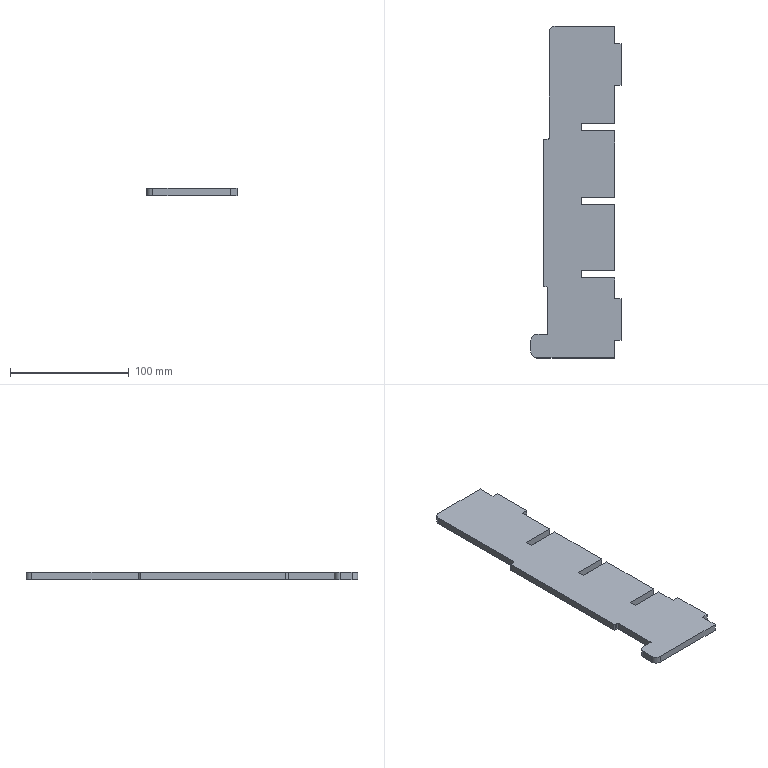Part | SolidWorks | features Fillet 1, FlatPattern 1, SMBaseFlange 1, SheetMetal 1 | 1 solid | 39 faces | box 76 x 280 x 6 mm | volume 97544 mm3 | plane 32 | cylinder 7 | commonest cylinder face diameters 2 x4 10 x3
STEP:
#1=CARTESIAN_POINT('',(-248.5,28.666,0.));
#2=VERTEX_POINT('',#1);
#3=CARTESIAN_POINT('',(-249.5,27.666,0.));
#4=VERTEX_POINT('',#3);
#5=CARTESIAN_POINT('',(-248.5,27.666,0.));
#6=DIRECTION('',(0.,0.,1.));
#7=DIRECTION('',(1.,0.,0.));
#8=AXIS2_PLACEMENT_3D('',#5,#6,#7);
#9=CIRCLE('',#8,1.);
#10=EDGE_CURVE('',#2,#4,#9,.T.);
#11=ORIENTED_EDGE('',*,*,#10,.F.);
#12=CARTESIAN_POINT('',(-248.5,28.666,-6.));
#13=VERTEX_POINT('',#12);
#14=CARTESIAN_POINT('',(-248.5,28.666,-6.));
#15=DIRECTION('',(0.,0.,1.));
#16=VECTOR('',#15,1000.);
#17=LINE('',#14,#16);
#18=EDGE_CURVE('',#13,#2,#17,.T.);
#19=ORIENTED_EDGE('',*,*,#18,.F.);
#20=CARTESIAN_POINT('',(-249.5,27.666,-6.));
#21=VERTEX_POINT('',#20);
#22=CARTESIAN_POINT('',(-248.5,27.666,-6.));
#23=DIRECTION('',(0.,0.,1.));
#24=DIRECTION('',(1.,0.,0.));
#25=AXIS2_PLACEMENT_3D('',#22,#23,#24);
#26=CIRCLE('',#25,1.);
#27=EDGE_CURVE('',#13,#21,#26,.T.);
#28=ORIENTED_EDGE('',*,*,#27,.T.);
#29=CARTESIAN_POINT('',(-249.5,27.666,-6.));
#30=DIRECTION('',(0.,0.,1.));
#31=VECTOR('',#30,1000.);
#32=LINE('',#29,#31);
#33=EDGE_CURVE('',#21,#4,#32,.T.);
#34=ORIENTED_EDGE('',*,*,#33,.T.);
#35=EDGE_LOOP('',(#11,#19,#28,#34));
#36=FACE_OUTER_BOUND('',#35,.T.);
#37=CARTESIAN_POINT('',(-248.5,27.666,-6.));
#38=DIRECTION('',(0.,0.,1.));
#39=DIRECTION('',(1.,0.,0.));
#40=AXIS2_PLACEMENT_3D('',#37,#38,#39);
#41=CYLINDRICAL_SURFACE('',#40,1.);
#42=ADVANCED_FACE('',(#36),#41,.T.);
#43=CARTESIAN_POINT('',(-245.5,28.666,0.));
#44=VERTEX_POINT('',#43);
#45=CARTESIAN_POINT('',(-248.5,28.666,0.));
#46=DIRECTION('',(-1.,0.,0.));
#47=VECTOR('',#46,1000.);
#48=LINE('',#45,#47);
#49=EDGE_CURVE('',#44,#2,#48,.T.);
#50=ORIENTED_EDGE('',*,*,#49,.F.);
#51=CARTESIAN_POINT('',(-245.5,28.666,-6.));
#52=VERTEX_POINT('',#51);
#53=CARTESIAN_POINT('',(-245.5,28.666,-6.));
#54=DIRECTION('',(0.,0.,1.));
#55=VECTOR('',#54,1000.);
#56=LINE('',#53,#55);
#57=EDGE_CURVE('',#52,#44,#56,.T.);
#58=ORIENTED_EDGE('',*,*,#57,.F.);
#59=CARTESIAN_POINT('',(-248.5,28.666,-6.));
#60=DIRECTION('',(-1.,0.,0.));
#61=VECTOR('',#60,1000.);
#62=LINE('',#59,#61);
#63=EDGE_CURVE('',#52,#13,#62,.T.);
#64=ORIENTED_EDGE('',*,*,#63,.T.);
#65=ORIENTED_EDGE('',*,*,#18,.T.);
#66=EDGE_LOOP('',(#50,#58,#64,#65));
#67=FACE_OUTER_BOUND('',#66,.T.);
#68=CARTESIAN_POINT('',(-248.5,28.666,-6.));
#69=DIRECTION('',(0.,1.,0.));
#70=DIRECTION('',(0.,0.,1.));
#71=AXIS2_PLACEMENT_3D('',#68,#69,#70);
#72=PLANE('',#71);
#73=ADVANCED_FACE('',(#67),#72,.T.);
#74=CARTESIAN_POINT('',(-244.5,29.666,0.));
#75=VERTEX_POINT('',#74);
#76=CARTESIAN_POINT('',(-245.5,29.666,0.));
#77=DIRECTION('',(0.,0.,-1.));
#78=DIRECTION('',(1.,0.,0.));
#79=AXIS2_PLACEMENT_3D('',#76,#77,#78);
#80=CIRCLE('',#79,1.);
#81=EDGE_CURVE('',#75,#44,#80,.T.);
#82=ORIENTED_EDGE('',*,*,#81,.F.);
#83=CARTESIAN_POINT('',(-244.5,29.666,-6.));
#84=VERTEX_POINT('',#83);
#85=CARTESIAN_POINT('',(-244.5,29.666,-6.));
#86=DIRECTION('',(0.,0.,1.));
#87=VECTOR('',#86,1000.);
#88=LINE('',#85,#87);
#89=EDGE_CURVE('',#84,#75,#88,.T.);
#90=ORIENTED_EDGE('',*,*,#89,.F.);
#91=CARTESIAN_POINT('',(-245.5,29.666,-6.));
#92=DIRECTION('',(0.,0.,-1.));
#93=DIRECTION('',(1.,0.,0.));
#94=AXIS2_PLACEMENT_3D('',#91,#92,#93);
#95=CIRCLE('',#94,1.);
#96=EDGE_CURVE('',#84,#52,#95,.T.);
#97=ORIENTED_EDGE('',*,*,#96,.T.);
#98=ORIENTED_EDGE('',*,*,#57,.T.);
#99=EDGE_LOOP('',(#82,#90,#97,#98));
#100=FACE_OUTER_BOUND('',#99,.T.);
#101=CARTESIAN_POINT('',(-245.5,29.666,-6.));
#102=DIRECTION('',(0.,0.,1.));
#103=DIRECTION('',(1.,0.,0.));
#104=AXIS2_PLACEMENT_3D('',#101,#102,#103);
#105=CYLINDRICAL_SURFACE('',#104,1.);
#106=ADVANCED_FACE('',(#100),#105,.F.);
#107=CARTESIAN_POINT('',(-244.5,119.166,0.));
#108=VERTEX_POINT('',#107);
#109=CARTESIAN_POINT('',(-244.5,124.166,0.));
#110=DIRECTION('',(0.,-1.,0.));
#111=VECTOR('',#110,1000.);
#112=LINE('',#109,#111);
#113=EDGE_CURVE('',#108,#75,#112,.T.);
#114=ORIENTED_EDGE('',*,*,#113,.F.);
#115=CARTESIAN_POINT('',(-244.5,119.166,-6.));
#116=VERTEX_POINT('',#115);
#117=CARTESIAN_POINT('',(-244.5,119.166,-6.));
#118=DIRECTION('',(0.,0.,-1.));
#119=VECTOR('',#118,1000.);
#120=LINE('',#117,#119);
#121=EDGE_CURVE('',#108,#116,#120,.T.);
#122=ORIENTED_EDGE('',*,*,#121,.T.);
#123=CARTESIAN_POINT('',(-244.5,124.166,-6.));
#124=DIRECTION('',(0.,-1.,0.));
#125=VECTOR('',#124,1000.);
#126=LINE('',#123,#125);
#127=EDGE_CURVE('',#116,#84,#126,.T.);
#128=ORIENTED_EDGE('',*,*,#127,.T.);
#129=ORIENTED_EDGE('',*,*,#89,.T.);
#130=EDGE_LOOP('',(#114,#122,#128,#129));
#131=FACE_OUTER_BOUND('',#130,.T.);
#132=CARTESIAN_POINT('',(-244.5,124.166,-6.));
#133=DIRECTION('',(-1.,0.,0.));
#134=DIRECTION('',(0.,-1.,0.));
#135=AXIS2_PLACEMENT_3D('',#132,#133,#134);
#136=PLANE('',#135);
#137=ADVANCED_FACE('',(#131),#136,.T.);
#138=CARTESIAN_POINT('',(-189.5,124.166,-6.));
#139=VERTEX_POINT('',#138);
#140=CARTESIAN_POINT('',(-239.5,124.166,-6.));
#141=VERTEX_POINT('',#140);
#142=CARTESIAN_POINT('',(-189.5,124.166,-6.));
#143=DIRECTION('',(-1.,0.,0.));
#144=VECTOR('',#143,1000.);
#145=LINE('',#142,#144);
#146=EDGE_CURVE('',#139,#141,#145,.T.);
#147=ORIENTED_EDGE('',*,*,#146,.T.);
#148=CARTESIAN_POINT('',(-239.5,124.166,0.));
#149=VERTEX_POINT('',#148);
#150=CARTESIAN_POINT('',(-239.5,124.166,-6.));
#151=DIRECTION('',(0.,0.,1.));
#152=VECTOR('',#151,1000.);
#153=LINE('',#150,#152);
#154=EDGE_CURVE('',#141,#149,#153,.T.);
#155=ORIENTED_EDGE('',*,*,#154,.T.);
#156=CARTESIAN_POINT('',(-189.5,124.166,0.));
#157=VERTEX_POINT('',#156);
#158=CARTESIAN_POINT('',(-189.5,124.166,0.));
#159=DIRECTION('',(-1.,0.,0.));
#160=VECTOR('',#159,1000.);
#161=LINE('',#158,#160);
#162=EDGE_CURVE('',#157,#149,#161,.T.);
#163=ORIENTED_EDGE('',*,*,#162,.F.);
#164=CARTESIAN_POINT('',(-189.5,124.166,-6.));
#165=DIRECTION('',(0.,0.,1.));
#166=VECTOR('',#165,1000.);
#167=LINE('',#164,#166);
#168=EDGE_CURVE('',#139,#157,#167,.T.);
#169=ORIENTED_EDGE('',*,*,#168,.F.);
#170=EDGE_LOOP('',(#147,#155,#163,#169));
#171=FACE_OUTER_BOUND('',#170,.T.);
#172=CARTESIAN_POINT('',(-189.5,124.166,-6.));
#173=DIRECTION('',(0.,1.,0.));
#174=DIRECTION('',(0.,0.,1.));
#175=AXIS2_PLACEMENT_3D('',#172,#173,#174);
#176=PLANE('',#175);
#177=ADVANCED_FACE('',(#171),#176,.T.);
#178=CARTESIAN_POINT('',(-189.5,109.166,0.));
#179=VERTEX_POINT('',#178);
#180=CARTESIAN_POINT('',(-189.5,109.166,0.));
#181=DIRECTION('',(0.,1.,0.));
#182=VECTOR('',#181,1000.);
#183=LINE('',#180,#182);
#184=EDGE_CURVE('',#179,#157,#183,.T.);
#185=ORIENTED_EDGE('',*,*,#184,.F.);
#186=CARTESIAN_POINT('',(-189.5,109.166,-6.));
#187=VERTEX_POINT('',#186);
#188=CARTESIAN_POINT('',(-189.5,109.166,-6.));
#189=DIRECTION('',(0.,0.,1.));
#190=VECTOR('',#189,1000.);
#191=LINE('',#188,#190);
#192=EDGE_CURVE('',#187,#179,#191,.T.);
#193=ORIENTED_EDGE('',*,*,#192,.F.);
#194=CARTESIAN_POINT('',(-189.5,109.166,-6.));
#195=DIRECTION('',(0.,1.,0.));
#196=VECTOR('',#195,1000.);
#197=LINE('',#194,#196);
#198=EDGE_CURVE('',#187,#139,#197,.T.);
#199=ORIENTED_EDGE('',*,*,#198,.T.);
#200=ORIENTED_EDGE('',*,*,#168,.T.);
#201=EDGE_LOOP('',(#185,#193,#199,#200));
#202=FACE_OUTER_BOUND('',#201,.T.);
#203=CARTESIAN_POINT('',(-189.5,109.166,-6.));
#204=DIRECTION('',(1.,0.,0.));
#205=DIRECTION('',(0.,1.,0.));
#206=AXIS2_PLACEMENT_3D('',#203,#204,#205);
#207=PLANE('',#206);
#208=ADVANCED_FACE('',(#202),#207,.T.);
#209=CARTESIAN_POINT('',(-184.,109.166,0.));
#210=VERTEX_POINT('',#209);
#211=CARTESIAN_POINT('',(-189.5,109.166,0.));
#212=DIRECTION('',(-1.,0.,0.));
#213=VECTOR('',#212,1000.);
#214=LINE('',#211,#213);
#215=EDGE_CURVE('',#210,#179,#214,.T.);
#216=ORIENTED_EDGE('',*,*,#215,.F.);
#217=CARTESIAN_POINT('',(-184.,109.166,-6.));
#218=VERTEX_POINT('',#217);
#219=CARTESIAN_POINT('',(-184.,109.166,-6.));
#220=DIRECTION('',(0.,0.,1.));
#221=VECTOR('',#220,1000.);
#222=LINE('',#219,#221);
#223=EDGE_CURVE('',#218,#210,#222,.T.);
#224=ORIENTED_EDGE('',*,*,#223,.F.);
#225=CARTESIAN_POINT('',(-189.5,109.166,-6.));
#226=DIRECTION('',(-1.,0.,0.));
#227=VECTOR('',#226,1000.);
#228=LINE('',#225,#227);
#229=EDGE_CURVE('',#218,#187,#228,.T.);
#230=ORIENTED_EDGE('',*,*,#229,.T.);
#231=ORIENTED_EDGE('',*,*,#192,.T.);
#232=EDGE_LOOP('',(#216,#224,#230,#231));
#233=FACE_OUTER_BOUND('',#232,.T.);
#234=CARTESIAN_POINT('',(-189.5,109.166,-6.));
#235=DIRECTION('',(0.,1.,0.));
#236=DIRECTION('',(0.,0.,1.));
#237=AXIS2_PLACEMENT_3D('',#234,#235,#236);
#238=PLANE('',#237);
#239=ADVANCED_FACE('',(#233),#238,.T.);
#240=CARTESIAN_POINT('',(-184.,74.166,0.));
#241=VERTEX_POINT('',#240);
#242=CARTESIAN_POINT('',(-184.,109.166,0.));
#243=DIRECTION('',(0.,1.,0.));
#244=VECTOR('',#243,1000.);
#245=LINE('',#242,#244);
#246=EDGE_CURVE('',#241,#210,#245,.T.);
#247=ORIENTED_EDGE('',*,*,#246,.F.);
#248=CARTESIAN_POINT('',(-184.,74.166,-6.));
#249=VERTEX_POINT('',#248);
#250=CARTESIAN_POINT('',(-184.,74.166,-6.));
#251=DIRECTION('',(0.,0.,1.));
#252=VECTOR('',#251,1000.);
#253=LINE('',#250,#252);
#254=EDGE_CURVE('',#249,#241,#253,.T.);
#255=ORIENTED_EDGE('',*,*,#254,.F.);
#256=CARTESIAN_POINT('',(-184.,109.166,-6.));
#257=DIRECTION('',(0.,1.,0.));
#258=VECTOR('',#257,1000.);
#259=LINE('',#256,#258);
#260=EDGE_CURVE('',#249,#218,#259,.T.);
#261=ORIENTED_EDGE('',*,*,#260,.T.);
#262=ORIENTED_EDGE('',*,*,#223,.T.);
#263=EDGE_LOOP('',(#247,#255,#261,#262));
#264=FACE_OUTER_BOUND('',#263,.T.);
#265=CARTESIAN_POINT('',(-184.,109.166,-6.));
#266=DIRECTION('',(1.,0.,0.));
#267=DIRECTION('',(0.,0.,-1.));
#268=AXIS2_PLACEMENT_3D('',#265,#266,#267);
#269=PLANE('',#268);
#270=ADVANCED_FACE('',(#264),#269,.T.);
#271=CARTESIAN_POINT('',(-189.5,74.166,0.));
#272=VERTEX_POINT('',#271);
#273=CARTESIAN_POINT('',(-184.,74.166,0.));
#274=DIRECTION('',(1.,0.,0.));
#275=VECTOR('',#274,1000.);
#276=LINE('',#273,#275);
#277=EDGE_CURVE('',#272,#241,#276,.T.);
#278=ORIENTED_EDGE('',*,*,#277,.F.);
#279=CARTESIAN_POINT('',(-189.5,74.166,-6.));
#280=VERTEX_POINT('',#279);
#281=CARTESIAN_POINT('',(-189.5,74.166,-6.));
#282=DIRECTION('',(0.,0.,1.));
#283=VECTOR('',#282,1000.);
#284=LINE('',#281,#283);
#285=EDGE_CURVE('',#280,#272,#284,.T.);
#286=ORIENTED_EDGE('',*,*,#285,.F.);
#287=CARTESIAN_POINT('',(-184.,74.166,-6.));
#288=DIRECTION('',(1.,0.,0.));
#289=VECTOR('',#288,1000.);
#290=LINE('',#287,#289);
#291=EDGE_CURVE('',#280,#249,#290,.T.);
#292=ORIENTED_EDGE('',*,*,#291,.T.);
#293=ORIENTED_EDGE('',*,*,#254,.T.);
#294=EDGE_LOOP('',(#278,#286,#292,#293));
#295=FACE_OUTER_BOUND('',#294,.T.);
#296=CARTESIAN_POINT('',(-184.,74.166,-6.));
#297=DIRECTION('',(0.,-1.,0.));
#298=DIRECTION('',(0.,0.,-1.));
#299=AXIS2_PLACEMENT_3D('',#296,#297,#298);
#300=PLANE('',#299);
#301=ADVANCED_FACE('',(#295),#300,.T.);
#302=CARTESIAN_POINT('',(-189.5,41.666,0.));
#303=VERTEX_POINT('',#302);
#304=CARTESIAN_POINT('',(-189.5,41.666,0.));
#305=DIRECTION('',(0.,1.,0.));
#306=VECTOR('',#305,1000.);
#307=LINE('',#304,#306);
#308=EDGE_CURVE('',#303,#272,#307,.T.);
#309=ORIENTED_EDGE('',*,*,#308,.F.);
#310=CARTESIAN_POINT('',(-189.5,41.666,-6.));
#311=VERTEX_POINT('',#310);
#312=CARTESIAN_POINT('',(-189.5,41.666,-6.));
#313=DIRECTION('',(0.,0.,1.));
#314=VECTOR('',#313,1000.);
#315=LINE('',#312,#314);
#316=EDGE_CURVE('',#311,#303,#315,.T.);
#317=ORIENTED_EDGE('',*,*,#316,.F.);
#318=CARTESIAN_POINT('',(-189.5,41.666,-6.));
#319=DIRECTION('',(0.,1.,0.));
#320=VECTOR('',#319,1000.);
#321=LINE('',#318,#320);
#322=EDGE_CURVE('',#311,#280,#321,.T.);
#323=ORIENTED_EDGE('',*,*,#322,.T.);
#324=ORIENTED_EDGE('',*,*,#285,.T.);
#325=EDGE_LOOP('',(#309,#317,#323,#324));
#326=FACE_OUTER_BOUND('',#325,.T.);
#327=CARTESIAN_POINT('',(-189.5,41.666,-6.));
#328=DIRECTION('',(1.,0.,0.));
#329=DIRECTION('',(0.,1.,0.));
#330=AXIS2_PLACEMENT_3D('',#327,#328,#329);
#331=PLANE('',#330);
#332=ADVANCED_FACE('',(#326),#331,.T.);
#333=CARTESIAN_POINT('',(-217.5,41.666,0.));
#334=VERTEX_POINT('',#333);
#335=CARTESIAN_POINT('',(-217.5,41.666,0.));
#336=DIRECTION('',(1.,0.,0.));
#337=VECTOR('',#336,1000.);
#338=LINE('',#335,#337);
#339=EDGE_CURVE('',#334,#303,#338,.T.);
#340=ORIENTED_EDGE('',*,*,#339,.F.);
#341=CARTESIAN_POINT('',(-217.5,41.666,-6.));
#342=VERTEX_POINT('',#341);
#343=CARTESIAN_POINT('',(-217.5,41.666,-6.));
#344=DIRECTION('',(0.,0.,1.));
#345=VECTOR('',#344,1000.);
#346=LINE('',#343,#345);
#347=EDGE_CURVE('',#342,#334,#346,.T.);
#348=ORIENTED_EDGE('',*,*,#347,.F.);
#349=CARTESIAN_POINT('',(-217.5,41.666,-6.));
#350=DIRECTION('',(1.,0.,0.));
#351=VECTOR('',#350,1000.);
#352=LINE('',#349,#351);
#353=EDGE_CURVE('',#342,#311,#352,.T.);
#354=ORIENTED_EDGE('',*,*,#353,.T.);
#355=ORIENTED_EDGE('',*,*,#316,.T.);
#356=EDGE_LOOP('',(#340,#348,#354,#355));
#357=FACE_OUTER_BOUND('',#356,.T.);
#358=CARTESIAN_POINT('',(-217.5,41.666,-6.));
#359=DIRECTION('',(0.,-1.,0.));
#360=DIRECTION('',(1.,0.,0.));
#361=AXIS2_PLACEMENT_3D('',#358,#359,#360);
#362=PLANE('',#361);
#363=ADVANCED_FACE('',(#357),#362,.T.);
#364=CARTESIAN_POINT('',(-217.5,35.666,0.));
#365=VERTEX_POINT('',#364);
#366=CARTESIAN_POINT('',(-217.5,35.666,0.));
#367=DIRECTION('',(0.,1.,0.));
#368=VECTOR('',#367,1000.);
#369=LINE('',#366,#368);
#370=EDGE_CURVE('',#365,#334,#369,.T.);
#371=ORIENTED_EDGE('',*,*,#370,.F.);
#372=CARTESIAN_POINT('',(-217.5,35.666,-6.));
#373=VERTEX_POINT('',#372);
#374=CARTESIAN_POINT('',(-217.5,35.666,-6.));
#375=DIRECTION('',(0.,0.,1.));
#376=VECTOR('',#375,1000.);
#377=LINE('',#374,#376);
#378=EDGE_CURVE('',#373,#365,#377,.T.);
#379=ORIENTED_EDGE('',*,*,#378,.F.);
#380=CARTESIAN_POINT('',(-217.5,35.666,-6.));
#381=DIRECTION('',(0.,1.,0.));
#382=VECTOR('',#381,1000.);
#383=LINE('',#380,#382);
#384=EDGE_CURVE('',#373,#342,#383,.T.);
#385=ORIENTED_EDGE('',*,*,#384,.T.);
#386=ORIENTED_EDGE('',*,*,#347,.T.);
#387=EDGE_LOOP('',(#371,#379,#385,#386));
#388=FACE_OUTER_BOUND('',#387,.T.);
#389=CARTESIAN_POINT('',(-217.5,35.666,-6.));
#390=DIRECTION('',(1.,0.,0.));
#391=DIRECTION('',(0.,0.,-1.));
#392=AXIS2_PLACEMENT_3D('',#389,#390,#391);
#393=PLANE('',#392);
#394=ADVANCED_FACE('',(#388),#393,.T.);
#395=CARTESIAN_POINT('',(-189.5,35.666,0.));
#396=VERTEX_POINT('',#395);
#397=CARTESIAN_POINT('',(-189.5,35.666,0.));
#398=DIRECTION('',(-1.,0.,0.));
#399=VECTOR('',#398,1000.);
#400=LINE('',#397,#399);
#401=EDGE_CURVE('',#396,#365,#400,.T.);
#402=ORIENTED_EDGE('',*,*,#401,.F.);
#403=CARTESIAN_POINT('',(-189.5,35.666,-6.));
#404=VERTEX_POINT('',#403);
#405=CARTESIAN_POINT('',(-189.5,35.666,-6.));
#406=DIRECTION('',(0.,0.,1.));
#407=VECTOR('',#406,1000.);
#408=LINE('',#405,#407);
#409=EDGE_CURVE('',#404,#396,#408,.T.);
#410=ORIENTED_EDGE('',*,*,#409,.F.);
#411=CARTESIAN_POINT('',(-189.5,35.666,-6.));
#412=DIRECTION('',(-1.,0.,0.));
#413=VECTOR('',#412,1000.);
#414=LINE('',#411,#413);
#415=EDGE_CURVE('',#404,#373,#414,.T.);
#416=ORIENTED_EDGE('',*,*,#415,.T.);
#417=ORIENTED_EDGE('',*,*,#378,.T.);
#418=EDGE_LOOP('',(#402,#410,#416,#417));
#419=FACE_OUTER_BOUND('',#418,.T.);
#420=CARTESIAN_POINT('',(-189.5,35.666,-6.));
#421=DIRECTION('',(0.,1.,0.));
#422=DIRECTION('',(-1.,0.,0.));
#423=AXIS2_PLACEMENT_3D('',#420,#421,#422);
#424=PLANE('',#423);
#425=ADVANCED_FACE('',(#419),#424,.T.);
#426=CARTESIAN_POINT('',(-189.5,-20.334,0.));
#427=VERTEX_POINT('',#426);
#428=CARTESIAN_POINT('',(-189.5,-20.334,0.));
#429=DIRECTION('',(0.,1.,0.));
#430=VECTOR('',#429,1000.);
#431=LINE('',#428,#430);
#432=EDGE_CURVE('',#427,#396,#431,.T.);
#433=ORIENTED_EDGE('',*,*,#432,.F.);
#434=CARTESIAN_POINT('',(-189.5,-20.334,-6.));
#435=VERTEX_POINT('',#434);
#436=CARTESIAN_POINT('',(-189.5,-20.334,-6.));
#437=DIRECTION('',(0.,0.,1.));
#438=VECTOR('',#437,1000.);
#439=LINE('',#436,#438);
#440=EDGE_CURVE('',#435,#427,#439,.T.);
#441=ORIENTED_EDGE('',*,*,#440,.F.);
#442=CARTESIAN_POINT('',(-189.5,-20.334,-6.));
#443=DIRECTION('',(0.,1.,0.));
#444=VECTOR('',#443,1000.);
#445=LINE('',#442,#444);
#446=EDGE_CURVE('',#435,#404,#445,.T.);
#447=ORIENTED_EDGE('',*,*,#446,.T.);
#448=ORIENTED_EDGE('',*,*,#409,.T.);
#449=EDGE_LOOP('',(#433,#441,#447,#448));
#450=FACE_OUTER_BOUND('',#449,.T.);
#451=CARTESIAN_POINT('',(-189.5,-20.334,-6.));
#452=DIRECTION('',(1.,0.,0.));
#453=DIRECTION('',(0.,0.,-1.));
#454=AXIS2_PLACEMENT_3D('',#451,#452,#453);
#455=PLANE('',#454);
#456=ADVANCED_FACE('',(#450),#455,.T.);
#457=CARTESIAN_POINT('',(-217.5,-20.334,0.));
#458=VERTEX_POINT('',#457);
#459=CARTESIAN_POINT('',(-217.5,-20.334,0.));
#460=DIRECTION('',(1.,0.,0.));
#461=VECTOR('',#460,1000.);
#462=LINE('',#459,#461);
#463=EDGE_CURVE('',#458,#427,#462,.T.);
#464=ORIENTED_EDGE('',*,*,#463,.F.);
#465=CARTESIAN_POINT('',(-217.5,-20.334,-6.));
#466=VERTEX_POINT('',#465);
#467=CARTESIAN_POINT('',(-217.5,-20.334,-6.));
#468=DIRECTION('',(0.,0.,1.));
#469=VECTOR('',#468,1000.);
#470=LINE('',#467,#469);
#471=EDGE_CURVE('',#466,#458,#470,.T.);
#472=ORIENTED_EDGE('',*,*,#471,.F.);
#473=CARTESIAN_POINT('',(-217.5,-20.334,-6.));
#474=DIRECTION('',(1.,0.,0.));
#475=VECTOR('',#474,1000.);
#476=LINE('',#473,#475);
#477=EDGE_CURVE('',#466,#435,#476,.T.);
#478=ORIENTED_EDGE('',*,*,#477,.T.);
#479=ORIENTED_EDGE('',*,*,#440,.T.);
#480=EDGE_LOOP('',(#464,#472,#478,#479));
#481=FACE_OUTER_BOUND('',#480,.T.);
#482=CARTESIAN_POINT('',(-217.5,-20.334,-6.));
#483=DIRECTION('',(0.,-1.,0.));
#484=DIRECTION('',(1.,0.,0.));
#485=AXIS2_PLACEMENT_3D('',#482,#483,#484);
#486=PLANE('',#485);
#487=ADVANCED_FACE('',(#481),#486,.T.);
#488=CARTESIAN_POINT('',(-217.5,-26.334,0.));
#489=VERTEX_POINT('',#488);
#490=CARTESIAN_POINT('',(-217.5,-26.334,0.));
#491=DIRECTION('',(0.,1.,0.));
#492=VECTOR('',#491,1000.);
#493=LINE('',#490,#492);
#494=EDGE_CURVE('',#489,#458,#493,.T.);
#495=ORIENTED_EDGE('',*,*,#494,.F.);
#496=CARTESIAN_POINT('',(-217.5,-26.334,-6.));
#497=VERTEX_POINT('',#496);
#498=CARTESIAN_POINT('',(-217.5,-26.334,-6.));
#499=DIRECTION('',(0.,0.,1.));
#500=VECTOR('',#499,1000.);
#501=LINE('',#498,#500);
#502=EDGE_CURVE('',#497,#489,#501,.T.);
#503=ORIENTED_EDGE('',*,*,#502,.F.);
#504=CARTESIAN_POINT('',(-217.5,-26.334,-6.));
#505=DIRECTION('',(0.,1.,0.));
#506=VECTOR('',#505,1000.);
#507=LINE('',#504,#506);
#508=EDGE_CURVE('',#497,#466,#507,.T.);
#509=ORIENTED_EDGE('',*,*,#508,.T.);
#510=ORIENTED_EDGE('',*,*,#471,.T.);
#511=EDGE_LOOP('',(#495,#503,#509,#510));
#512=FACE_OUTER_BOUND('',#511,.T.);
#513=CARTESIAN_POINT('',(-217.5,-26.334,-6.));
#514=DIRECTION('',(1.,0.,0.));
#515=DIRECTION('',(0.,0.,-1.));
#516=AXIS2_PLACEMENT_3D('',#513,#514,#515);
#517=PLANE('',#516);
#518=ADVANCED_FACE('',(#512),#517,.T.);
#519=CARTESIAN_POINT('',(-189.5,-26.334,0.));
#520=VERTEX_POINT('',#519);
#521=CARTESIAN_POINT('',(-189.5,-26.334,0.));
#522=DIRECTION('',(-1.,0.,0.));
#523=VECTOR('',#522,1000.);
#524=LINE('',#521,#523);
#525=EDGE_CURVE('',#520,#489,#524,.T.);
#526=ORIENTED_EDGE('',*,*,#525,.F.);
#527=CARTESIAN_POINT('',(-189.5,-26.334,-6.));
#528=VERTEX_POINT('',#527);
#529=CARTESIAN_POINT('',(-189.5,-26.334,-6.));
#530=DIRECTION('',(0.,0.,1.));
#531=VECTOR('',#530,1000.);
#532=LINE('',#529,#531);
#533=EDGE_CURVE('',#528,#520,#532,.T.);
#534=ORIENTED_EDGE('',*,*,#533,.F.);
#535=CARTESIAN_POINT('',(-189.5,-26.334,-6.));
#536=DIRECTION('',(-1.,0.,0.));
#537=VECTOR('',#536,1000.);
#538=LINE('',#535,#537);
#539=EDGE_CURVE('',#528,#497,#538,.T.);
#540=ORIENTED_EDGE('',*,*,#539,.T.);
#541=ORIENTED_EDGE('',*,*,#502,.T.);
#542=EDGE_LOOP('',(#526,#534,#540,#541));
#543=FACE_OUTER_BOUND('',#542,.T.);
#544=CARTESIAN_POINT('',(-189.5,-26.334,-6.));
#545=DIRECTION('',(0.,1.,0.));
#546=DIRECTION('',(-1.,0.,0.));
#547=AXIS2_PLACEMENT_3D('',#544,#545,#546);
#548=PLANE('',#547);
#549=ADVANCED_FACE('',(#543),#548,.T.);
#550=CARTESIAN_POINT('',(-189.5,-82.334,0.));
#551=VERTEX_POINT('',#550);
#552=CARTESIAN_POINT('',(-189.5,-82.334,0.));
#553=DIRECTION('',(0.,1.,0.));
#554=VECTOR('',#553,1000.);
#555=LINE('',#552,#554);
#556=EDGE_CURVE('',#551,#520,#555,.T.);
#557=ORIENTED_EDGE('',*,*,#556,.F.);
#558=CARTESIAN_POINT('',(-189.5,-82.334,-6.));
#559=VERTEX_POINT('',#558);
#560=CARTESIAN_POINT('',(-189.5,-82.334,-6.));
#561=DIRECTION('',(0.,0.,1.));
#562=VECTOR('',#561,1000.);
#563=LINE('',#560,#562);
#564=EDGE_CURVE('',#559,#551,#563,.T.);
#565=ORIENTED_EDGE('',*,*,#564,.F.);
#566=CARTESIAN_POINT('',(-189.5,-82.334,-6.));
#567=DIRECTION('',(0.,1.,0.));
#568=VECTOR('',#567,1000.);
#569=LINE('',#566,#568);
#570=EDGE_CURVE('',#559,#528,#569,.T.);
#571=ORIENTED_EDGE('',*,*,#570,.T.);
#572=ORIENTED_EDGE('',*,*,#533,.T.);
#573=EDGE_LOOP('',(#557,#565,#571,#572));
#574=FACE_OUTER_BOUND('',#573,.T.);
#575=CARTESIAN_POINT('',(-189.5,-82.334,-6.));
#576=DIRECTION('',(1.,0.,0.));
#577=DIRECTION('',(0.,0.,-1.));
#578=AXIS2_PLACEMENT_3D('',#575,#576,#577);
#579=PLANE('',#578);
#580=ADVANCED_FACE('',(#574),#579,.T.);
#581=CARTESIAN_POINT('',(-217.5,-82.334,0.));
#582=VERTEX_POINT('',#581);
#583=CARTESIAN_POINT('',(-217.5,-82.334,0.));
#584=DIRECTION('',(1.,0.,0.));
#585=VECTOR('',#584,1000.);
#586=LINE('',#583,#585);
#587=EDGE_CURVE('',#582,#551,#586,.T.);
#588=ORIENTED_EDGE('',*,*,#587,.F.);
#589=CARTESIAN_POINT('',(-217.5,-82.334,-6.));
#590=VERTEX_POINT('',#589);
#591=CARTESIAN_POINT('',(-217.5,-82.334,-6.));
#592=DIRECTION('',(0.,0.,1.));
#593=VECTOR('',#592,1000.);
#594=LINE('',#591,#593);
#595=EDGE_CURVE('',#590,#582,#594,.T.);
#596=ORIENTED_EDGE('',*,*,#595,.F.);
#597=CARTESIAN_POINT('',(-217.5,-82.334,-6.));
#598=DIRECTION('',(1.,0.,0.));
#599=VECTOR('',#598,1000.);
#600=LINE('',#597,#599);
#601=EDGE_CURVE('',#590,#559,#600,.T.);
#602=ORIENTED_EDGE('',*,*,#601,.T.);
#603=ORIENTED_EDGE('',*,*,#564,.T.);
#604=EDGE_LOOP('',(#588,#596,#602,#603));
#605=FACE_OUTER_BOUND('',#604,.T.);
#606=CARTESIAN_POINT('',(-217.5,-82.334,-6.));
#607=DIRECTION('',(0.,-1.,0.));
#608=DIRECTION('',(1.,0.,0.));
#609=AXIS2_PLACEMENT_3D('',#606,#607,#608);
#610=PLANE('',#609);
#611=ADVANCED_FACE('',(#605),#610,.T.);
#612=CARTESIAN_POINT('',(-217.5,-88.334,0.));
#613=VERTEX_POINT('',#612);
#614=CARTESIAN_POINT('',(-217.5,-88.334,0.));
#615=DIRECTION('',(0.,1.,0.));
#616=VECTOR('',#615,1000.);
#617=LINE('',#614,#616);
#618=EDGE_CURVE('',#613,#582,#617,.T.);
#619=ORIENTED_EDGE('',*,*,#618,.F.);
#620=CARTESIAN_POINT('',(-217.5,-88.334,-6.));
#621=VERTEX_POINT('',#620);
#622=CARTESIAN_POINT('',(-217.5,-88.334,-6.));
#623=DIRECTION('',(0.,0.,1.));
#624=VECTOR('',#623,1000.);
#625=LINE('',#622,#624);
#626=EDGE_CURVE('',#621,#613,#625,.T.);
#627=ORIENTED_EDGE('',*,*,#626,.F.);
#628=CARTESIAN_POINT('',(-217.5,-88.334,-6.));
#629=DIRECTION('',(0.,1.,0.));
#630=VECTOR('',#629,1000.);
#631=LINE('',#628,#630);
#632=EDGE_CURVE('',#621,#590,#631,.T.);
#633=ORIENTED_EDGE('',*,*,#632,.T.);
#634=ORIENTED_EDGE('',*,*,#595,.T.);
#635=EDGE_LOOP('',(#619,#627,#633,#634));
#636=FACE_OUTER_BOUND('',#635,.T.);
#637=CARTESIAN_POINT('',(-217.5,-88.334,-6.));
#638=DIRECTION('',(1.,0.,0.));
#639=DIRECTION('',(0.,0.,-1.));
#640=AXIS2_PLACEMENT_3D('',#637,#638,#639);
#641=PLANE('',#640);
#642=ADVANCED_FACE('',(#636),#641,.T.);
#643=CARTESIAN_POINT('',(-189.5,-88.334,0.));
#644=VERTEX_POINT('',#643);
#645=CARTESIAN_POINT('',(-189.5,-88.334,0.));
#646=DIRECTION('',(-1.,0.,0.));
#647=VECTOR('',#646,1000.);
#648=LINE('',#645,#647);
#649=EDGE_CURVE('',#644,#613,#648,.T.);
#650=ORIENTED_EDGE('',*,*,#649,.F.);
#651=CARTESIAN_POINT('',(-189.5,-88.334,-6.));
#652=VERTEX_POINT('',#651);
#653=CARTESIAN_POINT('',(-189.5,-88.334,-6.));
#654=DIRECTION('',(0.,0.,1.));
#655=VECTOR('',#654,1000.);
#656=LINE('',#653,#655);
#657=EDGE_CURVE('',#652,#644,#656,.T.);
#658=ORIENTED_EDGE('',*,*,#657,.F.);
#659=CARTESIAN_POINT('',(-189.5,-88.334,-6.));
#660=DIRECTION('',(-1.,0.,0.));
#661=VECTOR('',#660,1000.);
#662=LINE('',#659,#661);
#663=EDGE_CURVE('',#652,#621,#662,.T.);
#664=ORIENTED_EDGE('',*,*,#663,.T.);
#665=ORIENTED_EDGE('',*,*,#626,.T.);
#666=EDGE_LOOP('',(#650,#658,#664,#665));
#667=FACE_OUTER_BOUND('',#666,.T.);
#668=CARTESIAN_POINT('',(-189.5,-88.334,-6.));
#669=DIRECTION('',(0.,1.,0.));
#670=DIRECTION('',(-1.,0.,0.));
#671=AXIS2_PLACEMENT_3D('',#668,#669,#670);
#672=PLANE('',#671);
#673=ADVANCED_FACE('',(#667),#672,.T.);
#674=CARTESIAN_POINT('',(-189.5,-105.834,0.));
#675=VERTEX_POINT('',#674);
#676=CARTESIAN_POINT('',(-189.5,-105.834,0.));
#677=DIRECTION('',(0.,1.,0.));
#678=VECTOR('',#677,1000.);
#679=LINE('',#676,#678);
#680=EDGE_CURVE('',#675,#644,#679,.T.);
#681=ORIENTED_EDGE('',*,*,#680,.F.);
#682=CARTESIAN_POINT('',(-189.5,-105.834,-6.));
#683=VERTEX_POINT('',#682);
#684=CARTESIAN_POINT('',(-189.5,-105.834,-6.));
#685=DIRECTION('',(0.,0.,1.));
#686=VECTOR('',#685,1000.);
#687=LINE('',#684,#686);
#688=EDGE_CURVE('',#683,#675,#687,.T.);
#689=ORIENTED_EDGE('',*,*,#688,.F.);
#690=CARTESIAN_POINT('',(-189.5,-105.834,-6.));
#691=DIRECTION('',(0.,1.,0.));
#692=VECTOR('',#691,1000.);
#693=LINE('',#690,#692);
#694=EDGE_CURVE('',#683,#652,#693,.T.);
#695=ORIENTED_EDGE('',*,*,#694,.T.);
#696=ORIENTED_EDGE('',*,*,#657,.T.);
#697=EDGE_LOOP('',(#681,#689,#695,#696));
#698=FACE_OUTER_BOUND('',#697,.T.);
#699=CARTESIAN_POINT('',(-189.5,-105.834,-6.));
#700=DIRECTION('',(1.,0.,0.));
#701=DIRECTION('',(0.,1.,0.));
#702=AXIS2_PLACEMENT_3D('',#699,#700,#701);
#703=PLANE('',#702);
#704=ADVANCED_FACE('',(#698),#703,.T.);
#705=CARTESIAN_POINT('',(-184.,-105.834,0.));
#706=VERTEX_POINT('',#705);
#707=CARTESIAN_POINT('',(-184.,-105.834,0.));
#708=DIRECTION('',(-1.,0.,0.));
#709=VECTOR('',#708,1000.);
#710=LINE('',#707,#709);
#711=EDGE_CURVE('',#706,#675,#710,.T.);
#712=ORIENTED_EDGE('',*,*,#711,.F.);
#713=CARTESIAN_POINT('',(-184.,-105.834,-6.));
#714=VERTEX_POINT('',#713);
#715=CARTESIAN_POINT('',(-184.,-105.834,-6.));
#716=DIRECTION('',(0.,0.,1.));
#717=VECTOR('',#716,1000.);
#718=LINE('',#715,#717);
#719=EDGE_CURVE('',#714,#706,#718,.T.);
#720=ORIENTED_EDGE('',*,*,#719,.F.);
#721=CARTESIAN_POINT('',(-184.,-105.834,-6.));
#722=DIRECTION('',(-1.,0.,0.));
#723=VECTOR('',#722,1000.);
#724=LINE('',#721,#723);
#725=EDGE_CURVE('',#714,#683,#724,.T.);
#726=ORIENTED_EDGE('',*,*,#725,.T.);
#727=ORIENTED_EDGE('',*,*,#688,.T.);
#728=EDGE_LOOP('',(#712,#720,#726,#727));
#729=FACE_OUTER_BOUND('',#728,.T.);
#730=CARTESIAN_POINT('',(-184.,-105.834,-6.));
#731=DIRECTION('',(0.,1.,0.));
#732=DIRECTION('',(0.,0.,1.));
#733=AXIS2_PLACEMENT_3D('',#730,#731,#732);
#734=PLANE('',#733);
#735=ADVANCED_FACE('',(#729),#734,.T.);
#736=CARTESIAN_POINT('',(-184.,-140.834,0.));
#737=VERTEX_POINT('',#736);
#738=CARTESIAN_POINT('',(-184.,-140.834,0.));
#739=DIRECTION('',(0.,1.,0.));
#740=VECTOR('',#739,1000.);
#741=LINE('',#738,#740);
#742=EDGE_CURVE('',#737,#706,#741,.T.);
#743=ORIENTED_EDGE('',*,*,#742,.F.);
#744=CARTESIAN_POINT('',(-184.,-140.834,-6.));
#745=VERTEX_POINT('',#744);
#746=CARTESIAN_POINT('',(-184.,-140.834,-6.));
#747=DIRECTION('',(0.,0.,1.));
#748=VECTOR('',#747,1000.);
#749=LINE('',#746,#748);
#750=EDGE_CURVE('',#745,#737,#749,.T.);
#751=ORIENTED_EDGE('',*,*,#750,.F.);
#752=CARTESIAN_POINT('',(-184.,-140.834,-6.));
#753=DIRECTION('',(0.,1.,0.));
#754=VECTOR('',#753,1000.);
#755=LINE('',#752,#754);
#756=EDGE_CURVE('',#745,#714,#755,.T.);
#757=ORIENTED_EDGE('',*,*,#756,.T.);
#758=ORIENTED_EDGE('',*,*,#719,.T.);
#759=EDGE_LOOP('',(#743,#751,#757,#758));
#760=FACE_OUTER_BOUND('',#759,.T.);
#761=CARTESIAN_POINT('',(-184.,-140.834,-6.));
#762=DIRECTION('',(1.,0.,0.));
#763=DIRECTION('',(0.,0.,-1.));
#764=AXIS2_PLACEMENT_3D('',#761,#762,#763);
#765=PLANE('',#764);
#766=ADVANCED_FACE('',(#760),#765,.T.);
#767=CARTESIAN_POINT('',(-189.5,-140.834,0.));
#768=VERTEX_POINT('',#767);
#769=CARTESIAN_POINT('',(-189.5,-140.834,0.));
#770=DIRECTION('',(1.,0.,0.));
#771=VECTOR('',#770,1000.);
#772=LINE('',#769,#771);
#773=EDGE_CURVE('',#768,#737,#772,.T.);
#774=ORIENTED_EDGE('',*,*,#773,.F.);
#775=CARTESIAN_POINT('',(-189.5,-140.834,-6.));
#776=VERTEX_POINT('',#775);
#777=CARTESIAN_POINT('',(-189.5,-140.834,-6.));
#778=DIRECTION('',(0.,0.,1.));
#779=VECTOR('',#778,1000.);
#780=LINE('',#777,#779);
#781=EDGE_CURVE('',#776,#768,#780,.T.);
#782=ORIENTED_EDGE('',*,*,#781,.F.);
#783=CARTESIAN_POINT('',(-189.5,-140.834,-6.));
#784=DIRECTION('',(1.,0.,0.));
#785=VECTOR('',#784,1000.);
#786=LINE('',#783,#785);
#787=EDGE_CURVE('',#776,#745,#786,.T.);
#788=ORIENTED_EDGE('',*,*,#787,.T.);
#789=ORIENTED_EDGE('',*,*,#750,.T.);
#790=EDGE_LOOP('',(#774,#782,#788,#789));
#791=FACE_OUTER_BOUND('',#790,.T.);
#792=CARTESIAN_POINT('',(-189.5,-140.834,-6.));
#793=DIRECTION('',(0.,-1.,0.));
#794=DIRECTION('',(0.,0.,-1.));
#795=AXIS2_PLACEMENT_3D('',#792,#793,#794);
#796=PLANE('',#795);
#797=ADVANCED_FACE('',(#791),#796,.T.);
#798=CARTESIAN_POINT('',(-189.5,-155.834,0.));
#799=VERTEX_POINT('',#798);
#800=CARTESIAN_POINT('',(-189.5,-155.834,0.));
#801=DIRECTION('',(0.,1.,0.));
#802=VECTOR('',#801,1000.);
#803=LINE('',#800,#802);
#804=EDGE_CURVE('',#799,#768,#803,.T.);
#805=ORIENTED_EDGE('',*,*,#804,.F.);
#806=CARTESIAN_POINT('',(-189.5,-155.834,-6.));
#807=VERTEX_POINT('',#806);
#808=CARTESIAN_POINT('',(-189.5,-155.834,-6.));
#809=DIRECTION('',(0.,0.,1.));
#810=VECTOR('',#809,1000.);
#811=LINE('',#808,#810);
#812=EDGE_CURVE('',#807,#799,#811,.T.);
#813=ORIENTED_EDGE('',*,*,#812,.F.);
#814=CARTESIAN_POINT('',(-189.5,-155.834,-6.));
#815=DIRECTION('',(0.,1.,0.));
#816=VECTOR('',#815,1000.);
#817=LINE('',#814,#816);
#818=EDGE_CURVE('',#807,#776,#817,.T.);
#819=ORIENTED_EDGE('',*,*,#818,.T.);
#820=ORIENTED_EDGE('',*,*,#781,.T.);
#821=EDGE_LOOP('',(#805,#813,#819,#820));
#822=FACE_OUTER_BOUND('',#821,.T.);
#823=CARTESIAN_POINT('',(-189.5,-155.834,-6.));
#824=DIRECTION('',(1.,0.,0.));
#825=DIRECTION('',(0.,1.,0.));
#826=AXIS2_PLACEMENT_3D('',#823,#824,#825);
#827=PLANE('',#826);
#828=ADVANCED_FACE('',(#822),#827,.T.);
#829=CARTESIAN_POINT('',(-255.,-155.834,0.));
#830=VERTEX_POINT('',#829);
#831=CARTESIAN_POINT('',(-260.,-155.834,0.));
#832=DIRECTION('',(1.,0.,0.));
#833=VECTOR('',#832,1000.);
#834=LINE('',#831,#833);
#835=EDGE_CURVE('',#830,#799,#834,.T.);
#836=ORIENTED_EDGE('',*,*,#835,.F.);
#837=CARTESIAN_POINT('',(-255.,-155.834,-6.));
#838=VERTEX_POINT('',#837);
#839=CARTESIAN_POINT('',(-255.,-155.834,-6.));
#840=DIRECTION('',(0.,0.,-1.));
#841=VECTOR('',#840,1000.);
#842=LINE('',#839,#841);
#843=EDGE_CURVE('',#830,#838,#842,.T.);
#844=ORIENTED_EDGE('',*,*,#843,.T.);
#845=CARTESIAN_POINT('',(-260.,-155.834,-6.));
#846=DIRECTION('',(1.,0.,0.));
#847=VECTOR('',#846,1000.);
#848=LINE('',#845,#847);
#849=EDGE_CURVE('',#838,#807,#848,.T.);
#850=ORIENTED_EDGE('',*,*,#849,.T.);
#851=ORIENTED_EDGE('',*,*,#812,.T.);
#852=EDGE_LOOP('',(#836,#844,#850,#851));
#853=FACE_OUTER_BOUND('',#852,.T.);
#854=CARTESIAN_POINT('',(-260.,-155.834,-6.));
#855=DIRECTION('',(0.,-1.,0.));
#856=DIRECTION('',(0.,0.,-1.));
#857=AXIS2_PLACEMENT_3D('',#854,#855,#856);
#858=PLANE('',#857);
#859=ADVANCED_FACE('',(#853),#858,.T.);
#860=CARTESIAN_POINT('',(-260.,-140.834,0.));
#861=VERTEX_POINT('',#860);
#862=CARTESIAN_POINT('',(-260.,-150.834,0.));
#863=VERTEX_POINT('',#862);
#864=CARTESIAN_POINT('',(-260.,-155.834,0.));
#865=DIRECTION('',(0.,-1.,0.));
#866=VECTOR('',#865,1000.);
#867=LINE('',#864,#866);
#868=EDGE_CURVE('',#861,#863,#867,.T.);
#869=ORIENTED_EDGE('',*,*,#868,.F.);
#870=CARTESIAN_POINT('',(-260.,-140.834,-6.));
#871=VERTEX_POINT('',#870);
#872=CARTESIAN_POINT('',(-260.,-140.834,-6.));
#873=DIRECTION('',(0.,0.,-1.));
#874=VECTOR('',#873,1000.);
#875=LINE('',#872,#874);
#876=EDGE_CURVE('',#861,#871,#875,.T.);
#877=ORIENTED_EDGE('',*,*,#876,.T.);
#878=CARTESIAN_POINT('',(-260.,-150.834,-6.));
#879=VERTEX_POINT('',#878);
#880=CARTESIAN_POINT('',(-260.,-155.834,-6.));
#881=DIRECTION('',(0.,-1.,0.));
#882=VECTOR('',#881,1000.);
#883=LINE('',#880,#882);
#884=EDGE_CURVE('',#871,#879,#883,.T.);
#885=ORIENTED_EDGE('',*,*,#884,.T.);
#886=CARTESIAN_POINT('',(-260.,-150.834,-6.));
#887=DIRECTION('',(0.,0.,1.));
#888=VECTOR('',#887,1000.);
#889=LINE('',#886,#888);
#890=EDGE_CURVE('',#879,#863,#889,.T.);
#891=ORIENTED_EDGE('',*,*,#890,.T.);
#892=EDGE_LOOP('',(#869,#877,#885,#891));
#893=FACE_OUTER_BOUND('',#892,.T.);
#894=CARTESIAN_POINT('',(-260.,-155.834,-6.));
#895=DIRECTION('',(-1.,0.,0.));
#896=DIRECTION('',(0.,-1.,0.));
#897=AXIS2_PLACEMENT_3D('',#894,#895,#896);
#898=PLANE('',#897);
#899=ADVANCED_FACE('',(#893),#898,.T.);
#900=CARTESIAN_POINT('',(-246.,-135.834,-6.));
#901=VERTEX_POINT('',#900);
#902=CARTESIAN_POINT('',(-255.,-135.834,-6.));
#903=VERTEX_POINT('',#902);
#904=CARTESIAN_POINT('',(-246.,-135.834,-6.));
#905=DIRECTION('',(-1.,0.,0.));
#906=VECTOR('',#905,1000.);
#907=LINE('',#904,#906);
#908=EDGE_CURVE('',#901,#903,#907,.T.);
#909=ORIENTED_EDGE('',*,*,#908,.T.);
#910=CARTESIAN_POINT('',(-255.,-135.834,0.));
#911=VERTEX_POINT('',#910);
#912=CARTESIAN_POINT('',(-255.,-135.834,-6.));
#913=DIRECTION('',(0.,0.,1.));
#914=VECTOR('',#913,1000.);
#915=LINE('',#912,#914);
#916=EDGE_CURVE('',#903,#911,#915,.T.);
#917=ORIENTED_EDGE('',*,*,#916,.T.);
#918=CARTESIAN_POINT('',(-246.,-135.834,0.));
#919=VERTEX_POINT('',#918);
#920=CARTESIAN_POINT('',(-246.,-135.834,0.));
#921=DIRECTION('',(-1.,0.,0.));
#922=VECTOR('',#921,1000.);
#923=LINE('',#920,#922);
#924=EDGE_CURVE('',#919,#911,#923,.T.);
#925=ORIENTED_EDGE('',*,*,#924,.F.);
#926=CARTESIAN_POINT('',(-246.,-135.834,-6.));
#927=DIRECTION('',(0.,0.,1.));
#928=VECTOR('',#927,1000.);
#929=LINE('',#926,#928);
#930=EDGE_CURVE('',#901,#919,#929,.T.);
#931=ORIENTED_EDGE('',*,*,#930,.F.);
#932=EDGE_LOOP('',(#909,#917,#925,#931));
#933=FACE_OUTER_BOUND('',#932,.T.);
#934=CARTESIAN_POINT('',(-246.,-135.834,-6.));
#935=DIRECTION('',(0.,1.,0.));
#936=DIRECTION('',(-1.,0.,0.));
#937=AXIS2_PLACEMENT_3D('',#934,#935,#936);
#938=PLANE('',#937);
#939=ADVANCED_FACE('',(#933),#938,.T.);
#940=CARTESIAN_POINT('',(-246.,-96.834,0.));
#941=VERTEX_POINT('',#940);
#942=CARTESIAN_POINT('',(-246.,-96.834,0.));
#943=DIRECTION('',(0.,-1.,0.));
#944=VECTOR('',#943,1000.);
#945=LINE('',#942,#944);
#946=EDGE_CURVE('',#941,#919,#945,.T.);
#947=ORIENTED_EDGE('',*,*,#946,.F.);
#948=CARTESIAN_POINT('',(-246.,-96.834,-6.));
#949=VERTEX_POINT('',#948);
#950=CARTESIAN_POINT('',(-246.,-96.834,-6.));
#951=DIRECTION('',(0.,0.,1.));
#952=VECTOR('',#951,1000.);
#953=LINE('',#950,#952);
#954=EDGE_CURVE('',#949,#941,#953,.T.);
#955=ORIENTED_EDGE('',*,*,#954,.F.);
#956=CARTESIAN_POINT('',(-246.,-96.834,-6.));
#957=DIRECTION('',(0.,-1.,0.));
#958=VECTOR('',#957,1000.);
#959=LINE('',#956,#958);
#960=EDGE_CURVE('',#949,#901,#959,.T.);
#961=ORIENTED_EDGE('',*,*,#960,.T.);
#962=ORIENTED_EDGE('',*,*,#930,.T.);
#963=EDGE_LOOP('',(#947,#955,#961,#962));
#964=FACE_OUTER_BOUND('',#963,.T.);
#965=CARTESIAN_POINT('',(-246.,-96.834,-6.));
#966=DIRECTION('',(-1.,0.,0.));
#967=DIRECTION('',(0.,-1.,0.));
#968=AXIS2_PLACEMENT_3D('',#965,#966,#967);
#969=PLANE('',#968);
#970=ADVANCED_FACE('',(#964),#969,.T.);
#971=CARTESIAN_POINT('',(-247.,-95.834,0.));
#972=VERTEX_POINT('',#971);
#973=CARTESIAN_POINT('',(-247.,-96.834,0.));
#974=DIRECTION('',(0.,0.,-1.));
#975=DIRECTION('',(-1.,0.,0.));
#976=AXIS2_PLACEMENT_3D('',#973,#974,#975);
#977=CIRCLE('',#976,1.);
#978=EDGE_CURVE('',#972,#941,#977,.T.);
#979=ORIENTED_EDGE('',*,*,#978,.F.);
#980=CARTESIAN_POINT('',(-247.,-95.834,-6.));
#981=VERTEX_POINT('',#980);
#982=CARTESIAN_POINT('',(-247.,-95.834,-6.));
#983=DIRECTION('',(0.,0.,1.));
#984=VECTOR('',#983,1000.);
#985=LINE('',#982,#984);
#986=EDGE_CURVE('',#981,#972,#985,.T.);
#987=ORIENTED_EDGE('',*,*,#986,.F.);
#988=CARTESIAN_POINT('',(-247.,-96.834,-6.));
#989=DIRECTION('',(0.,0.,-1.));
#990=DIRECTION('',(-1.,0.,0.));
#991=AXIS2_PLACEMENT_3D('',#988,#989,#990);
#992=CIRCLE('',#991,1.);
#993=EDGE_CURVE('',#981,#949,#992,.T.);
#994=ORIENTED_EDGE('',*,*,#993,.T.);
#995=ORIENTED_EDGE('',*,*,#954,.T.);
#996=EDGE_LOOP('',(#979,#987,#994,#995));
#997=FACE_OUTER_BOUND('',#996,.T.);
#998=CARTESIAN_POINT('',(-247.,-96.834,-6.));
#999=DIRECTION('',(0.,0.,1.));
#1000=DIRECTION('',(1.,0.,0.));
#1001=AXIS2_PLACEMENT_3D('',#998,#999,#1000);
#1002=CYLINDRICAL_SURFACE('',#1001,1.);
#1003=ADVANCED_FACE('',(#997),#1002,.F.);
#1004=CARTESIAN_POINT('',(-248.5,-95.834,0.));
#1005=VERTEX_POINT('',#1004);
#1006=CARTESIAN_POINT('',(-248.5,-95.834,0.));
#1007=DIRECTION('',(1.,0.,0.));
#1008=VECTOR('',#1007,1000.);
#1009=LINE('',#1006,#1008);
#1010=EDGE_CURVE('',#1005,#972,#1009,.T.);
#1011=ORIENTED_EDGE('',*,*,#1010,.F.);
#1012=CARTESIAN_POINT('',(-248.5,-95.834,-6.));
#1013=VERTEX_POINT('',#1012);
#1014=CARTESIAN_POINT('',(-248.5,-95.834,-6.));
#1015=DIRECTION('',(0.,0.,1.));
#1016=VECTOR('',#1015,1000.);
#1017=LINE('',#1014,#1016);
#1018=EDGE_CURVE('',#1013,#1005,#1017,.T.);
#1019=ORIENTED_EDGE('',*,*,#1018,.F.);
#1020=CARTESIAN_POINT('',(-248.5,-95.834,-6.));
#1021=DIRECTION('',(1.,0.,0.));
#1022=VECTOR('',#1021,1000.);
#1023=LINE('',#1020,#1022);
#1024=EDGE_CURVE('',#1013,#981,#1023,.T.);
#1025=ORIENTED_EDGE('',*,*,#1024,.T.);
#1026=ORIENTED_EDGE('',*,*,#986,.T.);
#1027=EDGE_LOOP('',(#1011,#1019,#1025,#1026));
#1028=FACE_OUTER_BOUND('',#1027,.T.);
#1029=CARTESIAN_POINT('',(-248.5,-95.834,-6.));
#1030=DIRECTION('',(0.,-1.,0.));
#1031=DIRECTION('',(0.,0.,-1.));
#1032=AXIS2_PLACEMENT_3D('',#1029,#1030,#1031);
#1033=PLANE('',#1032);
#1034=ADVANCED_FACE('',(#1028),#1033,.T.);
#1035=CARTESIAN_POINT('',(-249.5,-94.834,0.));
#1036=VERTEX_POINT('',#1035);
#1037=CARTESIAN_POINT('',(-248.5,-94.834,0.));
#1038=DIRECTION('',(0.,0.,1.));
#1039=DIRECTION('',(1.,0.,0.));
#1040=AXIS2_PLACEMENT_3D('',#1037,#1038,#1039);
#1041=CIRCLE('',#1040,1.);
#1042=EDGE_CURVE('',#1036,#1005,#1041,.T.);
#1043=ORIENTED_EDGE('',*,*,#1042,.F.);
#1044=CARTESIAN_POINT('',(-249.5,-94.834,-6.));
#1045=VERTEX_POINT('',#1044);
#1046=CARTESIAN_POINT('',(-249.5,-94.834,-6.));
#1047=DIRECTION('',(0.,0.,1.));
#1048=VECTOR('',#1047,1000.);
#1049=LINE('',#1046,#1048);
#1050=EDGE_CURVE('',#1045,#1036,#1049,.T.);
#1051=ORIENTED_EDGE('',*,*,#1050,.F.);
#1052=CARTESIAN_POINT('',(-248.5,-94.834,-6.));
#1053=DIRECTION('',(0.,0.,1.));
#1054=DIRECTION('',(1.,0.,0.));
#1055=AXIS2_PLACEMENT_3D('',#1052,#1053,#1054);
#1056=CIRCLE('',#1055,1.);
#1057=EDGE_CURVE('',#1045,#1013,#1056,.T.);
#1058=ORIENTED_EDGE('',*,*,#1057,.T.);
#1059=ORIENTED_EDGE('',*,*,#1018,.T.);
#1060=EDGE_LOOP('',(#1043,#1051,#1058,#1059));
#1061=FACE_OUTER_BOUND('',#1060,.T.);
#1062=CARTESIAN_POINT('',(-248.5,-94.834,-6.));
#1063=DIRECTION('',(0.,0.,1.));
#1064=DIRECTION('',(1.,0.,0.));
#1065=AXIS2_PLACEMENT_3D('',#1062,#1063,#1064);
#1066=CYLINDRICAL_SURFACE('',#1065,1.);
#1067=ADVANCED_FACE('',(#1061),#1066,.T.);
#1068=CARTESIAN_POINT('',(-249.5,27.666,0.));
#1069=DIRECTION('',(0.,-1.,0.));
#1070=VECTOR('',#1069,1000.);
#1071=LINE('',#1068,#1070);
#1072=EDGE_CURVE('',#4,#1036,#1071,.T.);
#1073=ORIENTED_EDGE('',*,*,#1072,.F.);
#1074=ORIENTED_EDGE('',*,*,#33,.F.);
#1075=CARTESIAN_POINT('',(-249.5,27.666,-6.));
#1076=DIRECTION('',(0.,-1.,0.));
#1077=VECTOR('',#1076,1000.);
#1078=LINE('',#1075,#1077);
#1079=EDGE_CURVE('',#21,#1045,#1078,.T.);
#1080=ORIENTED_EDGE('',*,*,#1079,.T.);
#1081=ORIENTED_EDGE('',*,*,#1050,.T.);
#1082=EDGE_LOOP('',(#1073,#1074,#1080,#1081));
#1083=FACE_OUTER_BOUND('',#1082,.T.);
#1084=CARTESIAN_POINT('',(-249.5,27.666,-6.));
#1085=DIRECTION('',(-1.,0.,0.));
#1086=DIRECTION('',(0.,-1.,0.));
#1087=AXIS2_PLACEMENT_3D('',#1084,#1085,#1086);
#1088=PLANE('',#1087);
#1089=ADVANCED_FACE('',(#1083),#1088,.T.);
#1090=ORIENTED_EDGE('',*,*,#884,.F.);
#1091=CARTESIAN_POINT('',(-255.,-140.834,-6.));
#1092=DIRECTION('',(0.,0.,-1.));
#1093=DIRECTION('',(1.,0.,0.));
#1094=AXIS2_PLACEMENT_3D('',#1091,#1092,#1093);
#1095=CIRCLE('',#1094,5.);
#1096=EDGE_CURVE('',#871,#903,#1095,.T.);
#1097=ORIENTED_EDGE('',*,*,#1096,.T.);
#1098=ORIENTED_EDGE('',*,*,#908,.F.);
#1099=ORIENTED_EDGE('',*,*,#960,.F.);
#1100=ORIENTED_EDGE('',*,*,#993,.F.);
#1101=ORIENTED_EDGE('',*,*,#1024,.F.);
#1102=ORIENTED_EDGE('',*,*,#1057,.F.);
#1103=ORIENTED_EDGE('',*,*,#1079,.F.);
#1104=ORIENTED_EDGE('',*,*,#27,.F.);
#1105=ORIENTED_EDGE('',*,*,#63,.F.);
#1106=ORIENTED_EDGE('',*,*,#96,.F.);
#1107=ORIENTED_EDGE('',*,*,#127,.F.);
#1108=CARTESIAN_POINT('',(-239.5,119.166,-6.));
#1109=DIRECTION('',(0.,0.,-1.));
#1110=DIRECTION('',(1.,0.,0.));
#1111=AXIS2_PLACEMENT_3D('',#1108,#1109,#1110);
#1112=CIRCLE('',#1111,5.);
#1113=EDGE_CURVE('',#116,#141,#1112,.T.);
#1114=ORIENTED_EDGE('',*,*,#1113,.T.);
#1115=ORIENTED_EDGE('',*,*,#146,.F.);
#1116=ORIENTED_EDGE('',*,*,#198,.F.);
#1117=ORIENTED_EDGE('',*,*,#229,.F.);
#1118=ORIENTED_EDGE('',*,*,#260,.F.);
#1119=ORIENTED_EDGE('',*,*,#291,.F.);
#1120=ORIENTED_EDGE('',*,*,#322,.F.);
#1121=ORIENTED_EDGE('',*,*,#353,.F.);
#1122=ORIENTED_EDGE('',*,*,#384,.F.);
#1123=ORIENTED_EDGE('',*,*,#415,.F.);
#1124=ORIENTED_EDGE('',*,*,#446,.F.);
#1125=ORIENTED_EDGE('',*,*,#477,.F.);
#1126=ORIENTED_EDGE('',*,*,#508,.F.);
#1127=ORIENTED_EDGE('',*,*,#539,.F.);
#1128=ORIENTED_EDGE('',*,*,#570,.F.);
#1129=ORIENTED_EDGE('',*,*,#601,.F.);
#1130=ORIENTED_EDGE('',*,*,#632,.F.);
#1131=ORIENTED_EDGE('',*,*,#663,.F.);
#1132=ORIENTED_EDGE('',*,*,#694,.F.);
#1133=ORIENTED_EDGE('',*,*,#725,.F.);
#1134=ORIENTED_EDGE('',*,*,#756,.F.);
#1135=ORIENTED_EDGE('',*,*,#787,.F.);
#1136=ORIENTED_EDGE('',*,*,#818,.F.);
#1137=ORIENTED_EDGE('',*,*,#849,.F.);
#1138=CARTESIAN_POINT('',(-255.,-150.834,-6.));
#1139=DIRECTION('',(0.,0.,-1.));
#1140=DIRECTION('',(1.,0.,0.));
#1141=AXIS2_PLACEMENT_3D('',#1138,#1139,#1140);
#1142=CIRCLE('',#1141,5.);
#1143=EDGE_CURVE('',#838,#879,#1142,.T.);
#1144=ORIENTED_EDGE('',*,*,#1143,.T.);
#1145=EDGE_LOOP('',(#1090,#1097,#1098,#1099,#1100,#1101,#1102,#1103,#1104,#1105,#1106,#1107,#1114,#1115,#1116,#1117,#1118,#1119,#1120,#1121,#1122,#1123,#1124,#1125,#1126,#1127,#1128,#1129,#1130,#1131,#1132,#1133,#1134,#1135,#1136,#1137,#1144));
#1146=FACE_OUTER_BOUND('',#1145,.T.);
#1147=CARTESIAN_POINT('',(-248.5,27.666,-6.));
#1148=DIRECTION('',(0.,0.,1.));
#1149=DIRECTION('',(1.,0.,0.));
#1150=AXIS2_PLACEMENT_3D('',#1147,#1148,#1149);
#1151=PLANE('',#1150);
#1152=ADVANCED_FACE('',(#1146),#1151,.F.);
#1153=ORIENTED_EDGE('',*,*,#924,.T.);
#1154=CARTESIAN_POINT('',(-255.,-140.834,0.));
#1155=DIRECTION('',(0.,0.,1.));
#1156=DIRECTION('',(1.,0.,0.));
#1157=AXIS2_PLACEMENT_3D('',#1154,#1155,#1156);
#1158=CIRCLE('',#1157,5.);
#1159=EDGE_CURVE('',#911,#861,#1158,.T.);
#1160=ORIENTED_EDGE('',*,*,#1159,.T.);
#1161=ORIENTED_EDGE('',*,*,#868,.T.);
#1162=CARTESIAN_POINT('',(-255.,-150.834,0.));
#1163=DIRECTION('',(0.,0.,1.));
#1164=DIRECTION('',(1.,0.,0.));
#1165=AXIS2_PLACEMENT_3D('',#1162,#1163,#1164);
#1166=CIRCLE('',#1165,5.);
#1167=EDGE_CURVE('',#863,#830,#1166,.T.);
#1168=ORIENTED_EDGE('',*,*,#1167,.T.);
#1169=ORIENTED_EDGE('',*,*,#835,.T.);
#1170=ORIENTED_EDGE('',*,*,#804,.T.);
#1171=ORIENTED_EDGE('',*,*,#773,.T.);
#1172=ORIENTED_EDGE('',*,*,#742,.T.);
#1173=ORIENTED_EDGE('',*,*,#711,.T.);
#1174=ORIENTED_EDGE('',*,*,#680,.T.);
#1175=ORIENTED_EDGE('',*,*,#649,.T.);
#1176=ORIENTED_EDGE('',*,*,#618,.T.);
#1177=ORIENTED_EDGE('',*,*,#587,.T.);
#1178=ORIENTED_EDGE('',*,*,#556,.T.);
#1179=ORIENTED_EDGE('',*,*,#525,.T.);
#1180=ORIENTED_EDGE('',*,*,#494,.T.);
#1181=ORIENTED_EDGE('',*,*,#463,.T.);
#1182=ORIENTED_EDGE('',*,*,#432,.T.);
#1183=ORIENTED_EDGE('',*,*,#401,.T.);
#1184=ORIENTED_EDGE('',*,*,#370,.T.);
#1185=ORIENTED_EDGE('',*,*,#339,.T.);
#1186=ORIENTED_EDGE('',*,*,#308,.T.);
#1187=ORIENTED_EDGE('',*,*,#277,.T.);
#1188=ORIENTED_EDGE('',*,*,#246,.T.);
#1189=ORIENTED_EDGE('',*,*,#215,.T.);
#1190=ORIENTED_EDGE('',*,*,#184,.T.);
#1191=ORIENTED_EDGE('',*,*,#162,.T.);
#1192=CARTESIAN_POINT('',(-239.5,119.166,0.));
#1193=DIRECTION('',(0.,0.,1.));
#1194=DIRECTION('',(1.,0.,0.));
#1195=AXIS2_PLACEMENT_3D('',#1192,#1193,#1194);
#1196=CIRCLE('',#1195,5.);
#1197=EDGE_CURVE('',#149,#108,#1196,.T.);
#1198=ORIENTED_EDGE('',*,*,#1197,.T.);
#1199=ORIENTED_EDGE('',*,*,#113,.T.);
#1200=ORIENTED_EDGE('',*,*,#81,.T.);
#1201=ORIENTED_EDGE('',*,*,#49,.T.);
#1202=ORIENTED_EDGE('',*,*,#10,.T.);
#1203=ORIENTED_EDGE('',*,*,#1072,.T.);
#1204=ORIENTED_EDGE('',*,*,#1042,.T.);
#1205=ORIENTED_EDGE('',*,*,#1010,.T.);
#1206=ORIENTED_EDGE('',*,*,#978,.T.);
#1207=ORIENTED_EDGE('',*,*,#946,.T.);
#1208=EDGE_LOOP('',(#1153,#1160,#1161,#1168,#1169,#1170,#1171,#1172,#1173,#1174,#1175,#1176,#1177,#1178,#1179,#1180,#1181,#1182,#1183,#1184,#1185,#1186,#1187,#1188,#1189,#1190,#1191,#1198,#1199,#1200,#1201,#1202,#1203,#1204,#1205,#1206,#1207));
#1209=FACE_OUTER_BOUND('',#1208,.T.);
#1210=CARTESIAN_POINT('',(-248.5,27.666,0.));
#1211=DIRECTION('',(0.,0.,1.));
#1212=DIRECTION('',(1.,0.,0.));
#1213=AXIS2_PLACEMENT_3D('',#1210,#1211,#1212);
#1214=PLANE('',#1213);
#1215=ADVANCED_FACE('',(#1209),#1214,.T.);
#1216=ORIENTED_EDGE('',*,*,#1096,.F.);
#1217=ORIENTED_EDGE('',*,*,#876,.F.);
#1218=ORIENTED_EDGE('',*,*,#1159,.F.);
#1219=ORIENTED_EDGE('',*,*,#916,.F.);
#1220=EDGE_LOOP('',(#1216,#1217,#1218,#1219));
#1221=FACE_OUTER_BOUND('',#1220,.T.);
#1222=CARTESIAN_POINT('',(-255.,-140.834,-6.));
#1223=DIRECTION('',(0.,0.,1.));
#1224=DIRECTION('',(1.,0.,0.));
#1225=AXIS2_PLACEMENT_3D('',#1222,#1223,#1224);
#1226=CYLINDRICAL_SURFACE('',#1225,5.);
#1227=ADVANCED_FACE('',(#1221),#1226,.T.);
#1228=ORIENTED_EDGE('',*,*,#1143,.F.);
#1229=ORIENTED_EDGE('',*,*,#843,.F.);
#1230=ORIENTED_EDGE('',*,*,#1167,.F.);
#1231=ORIENTED_EDGE('',*,*,#890,.F.);
#1232=EDGE_LOOP('',(#1228,#1229,#1230,#1231));
#1233=FACE_OUTER_BOUND('',#1232,.T.);
#1234=CARTESIAN_POINT('',(-255.,-150.834,-6.));
#1235=DIRECTION('',(0.,0.,1.));
#1236=DIRECTION('',(1.,0.,0.));
#1237=AXIS2_PLACEMENT_3D('',#1234,#1235,#1236);
#1238=CYLINDRICAL_SURFACE('',#1237,5.);
#1239=ADVANCED_FACE('',(#1233),#1238,.T.);
#1240=ORIENTED_EDGE('',*,*,#1113,.F.);
#1241=ORIENTED_EDGE('',*,*,#121,.F.);
#1242=ORIENTED_EDGE('',*,*,#1197,.F.);
#1243=ORIENTED_EDGE('',*,*,#154,.F.);
#1244=EDGE_LOOP('',(#1240,#1241,#1242,#1243));
#1245=FACE_OUTER_BOUND('',#1244,.T.);
#1246=CARTESIAN_POINT('',(-239.5,119.166,-6.));
#1247=DIRECTION('',(0.,0.,1.));
#1248=DIRECTION('',(1.,0.,0.));
#1249=AXIS2_PLACEMENT_3D('',#1246,#1247,#1248);
#1250=CYLINDRICAL_SURFACE('',#1249,5.);
#1251=ADVANCED_FACE('',(#1245),#1250,.T.);
#1252=CLOSED_SHELL('',(#42,#73,#106,#137,#177,#208,#239,#270,#301,#332,#363,#394,#425,#456,#487,#518,#549,#580,#611,#642,#673,#704,#735,#766,#797,#828,#859,#899,#939,#970,#1003,#1034,#1067,#1089,#1152,#1215,#1227,#1239,#1251));
#1253=MANIFOLD_SOLID_BREP('',#1252);
#1254=CARTESIAN_POINT('',(0.,0.,0.));
#1255=DIRECTION('',(0.,0.,1.));
#1256=DIRECTION('',(1.,0.,0.));
#1257=AXIS2_PLACEMENT_3D('',#1254,#1255,#1256);
#1258=(LENGTH_UNIT()NAMED_UNIT(*)SI_UNIT(.MILLI.,.METRE.));
#1259=UNCERTAINTY_MEASURE_WITH_UNIT(LENGTH_MEASURE(0.00001),#1258,'','');
#1260=(NAMED_UNIT(*)PLANE_ANGLE_UNIT()SI_UNIT($,.RADIAN.));
#1261=(NAMED_UNIT(*)SI_UNIT($,.STERADIAN.)SOLID_ANGLE_UNIT());
#1262=(GEOMETRIC_REPRESENTATION_CONTEXT(3)GLOBAL_UNCERTAINTY_ASSIGNED_CONTEXT((#1259))GLOBAL_UNIT_ASSIGNED_CONTEXT((#1258,#1260,#1261))REPRESENTATION_CONTEXT('',''));
#1263=ADVANCED_BREP_SHAPE_REPRESENTATION('',(#1253,#1257),#1262);